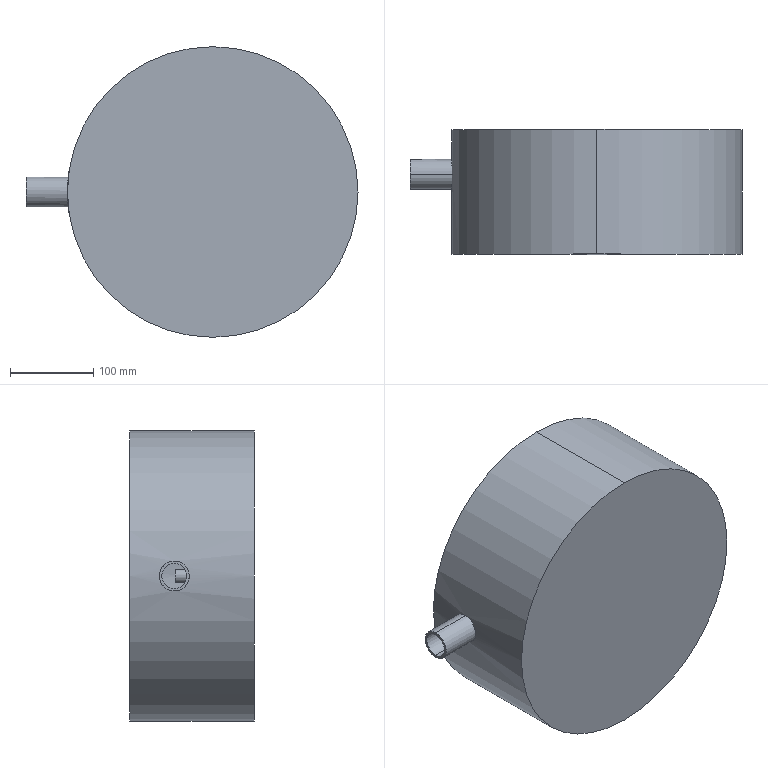Part | SolidWorks | features ICE 6, Extrusion 1, Shell 1 | 1 solid | 36 faces | box 400 x 150 x 350 mm | volume 1908298 mm3 | cylinder 24 | plane 12 | commonest cylinder face diameters 5 x8 36 x4 16 x2 30 x2 120 x2 320 x2
STEP:
#1=CARTESIAN_POINT('',(0.,145.,167.5));
#2=VERTEX_POINT('',#1);
#3=CARTESIAN_POINT('',(-2.5,145.,169.982));
#4=VERTEX_POINT('',#3);
#5=CARTESIAN_POINT('',(0.,145.,170.));
#6=DIRECTION('',(0.,1.,0.));
#7=DIRECTION('',(0.,0.,1.));
#8=AXIS2_PLACEMENT_3D('',#5,#6,#7);
#9=CIRCLE('',#8,2.5);
#10=EDGE_CURVE('',#2,#4,#9,.T.);
#11=ORIENTED_EDGE('',*,*,#10,.F.);
#12=CARTESIAN_POINT('',(0.,150.,167.5));
#13=VERTEX_POINT('',#12);
#14=CARTESIAN_POINT('',(0.,140.,167.5));
#15=DIRECTION('',(0.,1.,0.));
#16=VECTOR('',#15,1000.);
#17=LINE('',#14,#16);
#18=EDGE_CURVE('',#2,#13,#17,.T.);
#19=ORIENTED_EDGE('',*,*,#18,.T.);
#20=CARTESIAN_POINT('',(0.,150.,172.5));
#21=VERTEX_POINT('',#20);
#22=CARTESIAN_POINT('',(0.,150.,170.));
#23=DIRECTION('',(0.,1.,0.));
#24=DIRECTION('',(0.,0.,1.));
#25=AXIS2_PLACEMENT_3D('',#22,#23,#24);
#26=CIRCLE('',#25,2.5);
#27=EDGE_CURVE('',#13,#21,#26,.T.);
#28=ORIENTED_EDGE('',*,*,#27,.T.);
#29=CARTESIAN_POINT('',(0.,140.,172.5));
#30=VERTEX_POINT('',#29);
#31=CARTESIAN_POINT('',(0.,140.,172.5));
#32=DIRECTION('',(0.,1.,0.));
#33=VECTOR('',#32,1000.);
#34=LINE('',#31,#33);
#35=EDGE_CURVE('',#30,#21,#34,.T.);
#36=ORIENTED_EDGE('',*,*,#35,.F.);
#37=CARTESIAN_POINT('',(-2.5,140.,169.982));
#38=VERTEX_POINT('',#37);
#39=CARTESIAN_POINT('',(0.,140.,170.));
#40=DIRECTION('',(0.,1.,0.));
#41=DIRECTION('',(0.,0.,1.));
#42=AXIS2_PLACEMENT_3D('',#39,#40,#41);
#43=CIRCLE('',#42,2.5);
#44=EDGE_CURVE('',#38,#30,#43,.T.);
#45=ORIENTED_EDGE('',*,*,#44,.F.);
#46=CARTESIAN_POINT('',(-2.5,145.,169.982));
#47=DIRECTION('',(0.,1.,0.));
#48=VECTOR('',#47,1000.);
#49=LINE('',#46,#48);
#50=EDGE_CURVE('',#38,#4,#49,.T.);
#51=ORIENTED_EDGE('',*,*,#50,.T.);
#52=EDGE_LOOP('',(#11,#19,#28,#36,#45,#51));
#53=FACE_OUTER_BOUND('',#52,.T.);
#54=CARTESIAN_POINT('',(0.,140.,170.));
#55=DIRECTION('',(0.,1.,0.));
#56=DIRECTION('',(0.,0.,1.));
#57=AXIS2_PLACEMENT_3D('',#54,#55,#56);
#58=CYLINDRICAL_SURFACE('',#57,2.5);
#59=ADVANCED_FACE('',(#53),#58,.F.);
#60=CARTESIAN_POINT('',(-170.,140.,-2.5));
#61=VERTEX_POINT('',#60);
#62=CARTESIAN_POINT('',(-170.,140.,2.5));
#63=VERTEX_POINT('',#62);
#64=CARTESIAN_POINT('',(-170.,140.,0.));
#65=DIRECTION('',(0.,1.,0.));
#66=DIRECTION('',(0.,0.,1.));
#67=AXIS2_PLACEMENT_3D('',#64,#65,#66);
#68=CIRCLE('',#67,2.5);
#69=EDGE_CURVE('',#61,#63,#68,.T.);
#70=ORIENTED_EDGE('',*,*,#69,.F.);
#71=CARTESIAN_POINT('',(-170.,150.,-2.5));
#72=VERTEX_POINT('',#71);
#73=CARTESIAN_POINT('',(-170.,140.,-2.5));
#74=DIRECTION('',(0.,1.,0.));
#75=VECTOR('',#74,1000.);
#76=LINE('',#73,#75);
#77=EDGE_CURVE('',#61,#72,#76,.T.);
#78=ORIENTED_EDGE('',*,*,#77,.T.);
#79=CARTESIAN_POINT('',(-170.,150.,2.5));
#80=VERTEX_POINT('',#79);
#81=CARTESIAN_POINT('',(-170.,150.,0.));
#82=DIRECTION('',(0.,1.,0.));
#83=DIRECTION('',(0.,0.,1.));
#84=AXIS2_PLACEMENT_3D('',#81,#82,#83);
#85=CIRCLE('',#84,2.5);
#86=EDGE_CURVE('',#72,#80,#85,.T.);
#87=ORIENTED_EDGE('',*,*,#86,.T.);
#88=CARTESIAN_POINT('',(-170.,140.,2.5));
#89=DIRECTION('',(0.,1.,0.));
#90=VECTOR('',#89,1000.);
#91=LINE('',#88,#90);
#92=EDGE_CURVE('',#63,#80,#91,.T.);
#93=ORIENTED_EDGE('',*,*,#92,.F.);
#94=EDGE_LOOP('',(#70,#78,#87,#93));
#95=FACE_OUTER_BOUND('',#94,.T.);
#96=CARTESIAN_POINT('',(-170.,140.,0.));
#97=DIRECTION('',(0.,1.,0.));
#98=DIRECTION('',(0.,0.,1.));
#99=AXIS2_PLACEMENT_3D('',#96,#97,#98);
#100=CYLINDRICAL_SURFACE('',#99,2.5);
#101=ADVANCED_FACE('',(#95),#100,.F.);
#102=CARTESIAN_POINT('',(0.,140.,-172.5));
#103=VERTEX_POINT('',#102);
#104=CARTESIAN_POINT('',(-2.5,140.,-169.982));
#105=VERTEX_POINT('',#104);
#106=CARTESIAN_POINT('',(0.,140.,-170.));
#107=DIRECTION('',(0.,1.,0.));
#108=DIRECTION('',(0.,0.,1.));
#109=AXIS2_PLACEMENT_3D('',#106,#107,#108);
#110=CIRCLE('',#109,2.5);
#111=EDGE_CURVE('',#103,#105,#110,.T.);
#112=ORIENTED_EDGE('',*,*,#111,.F.);
#113=CARTESIAN_POINT('',(0.,150.,-172.5));
#114=VERTEX_POINT('',#113);
#115=CARTESIAN_POINT('',(0.,140.,-172.5));
#116=DIRECTION('',(0.,1.,0.));
#117=VECTOR('',#116,1000.);
#118=LINE('',#115,#117);
#119=EDGE_CURVE('',#103,#114,#118,.T.);
#120=ORIENTED_EDGE('',*,*,#119,.T.);
#121=CARTESIAN_POINT('',(0.,150.,-167.5));
#122=VERTEX_POINT('',#121);
#123=CARTESIAN_POINT('',(0.,150.,-170.));
#124=DIRECTION('',(0.,1.,0.));
#125=DIRECTION('',(0.,0.,1.));
#126=AXIS2_PLACEMENT_3D('',#123,#124,#125);
#127=CIRCLE('',#126,2.5);
#128=EDGE_CURVE('',#114,#122,#127,.T.);
#129=ORIENTED_EDGE('',*,*,#128,.T.);
#130=CARTESIAN_POINT('',(0.,145.,-167.5));
#131=VERTEX_POINT('',#130);
#132=CARTESIAN_POINT('',(0.,140.,-167.5));
#133=DIRECTION('',(0.,1.,0.));
#134=VECTOR('',#133,1000.);
#135=LINE('',#132,#134);
#136=EDGE_CURVE('',#131,#122,#135,.T.);
#137=ORIENTED_EDGE('',*,*,#136,.F.);
#138=CARTESIAN_POINT('',(-2.5,145.,-169.982));
#139=VERTEX_POINT('',#138);
#140=CARTESIAN_POINT('',(0.,145.,-170.));
#141=DIRECTION('',(0.,1.,0.));
#142=DIRECTION('',(0.,0.,1.));
#143=AXIS2_PLACEMENT_3D('',#140,#141,#142);
#144=CIRCLE('',#143,2.5);
#145=EDGE_CURVE('',#139,#131,#144,.T.);
#146=ORIENTED_EDGE('',*,*,#145,.F.);
#147=CARTESIAN_POINT('',(-2.5,145.,-169.982));
#148=DIRECTION('',(0.,-1.,0.));
#149=VECTOR('',#148,1000.);
#150=LINE('',#147,#149);
#151=EDGE_CURVE('',#139,#105,#150,.T.);
#152=ORIENTED_EDGE('',*,*,#151,.T.);
#153=EDGE_LOOP('',(#112,#120,#129,#137,#146,#152));
#154=FACE_OUTER_BOUND('',#153,.T.);
#155=CARTESIAN_POINT('',(0.,140.,-170.));
#156=DIRECTION('',(0.,1.,0.));
#157=DIRECTION('',(0.,0.,1.));
#158=AXIS2_PLACEMENT_3D('',#155,#156,#157);
#159=CYLINDRICAL_SURFACE('',#158,2.5);
#160=ADVANCED_FACE('',(#154),#159,.F.);
#161=CARTESIAN_POINT('',(170.,140.,-2.5));
#162=VERTEX_POINT('',#161);
#163=CARTESIAN_POINT('',(169.982,140.,-2.5));
#164=VERTEX_POINT('',#163);
#165=CARTESIAN_POINT('',(170.,140.,0.));
#166=DIRECTION('',(0.,1.,0.));
#167=DIRECTION('',(0.,0.,1.));
#168=AXIS2_PLACEMENT_3D('',#165,#166,#167);
#169=CIRCLE('',#168,2.5);
#170=EDGE_CURVE('',#162,#164,#169,.T.);
#171=ORIENTED_EDGE('',*,*,#170,.F.);
#172=CARTESIAN_POINT('',(170.,150.,-2.5));
#173=VERTEX_POINT('',#172);
#174=CARTESIAN_POINT('',(170.,140.,-2.5));
#175=DIRECTION('',(0.,1.,0.));
#176=VECTOR('',#175,1000.);
#177=LINE('',#174,#176);
#178=EDGE_CURVE('',#162,#173,#177,.T.);
#179=ORIENTED_EDGE('',*,*,#178,.T.);
#180=CARTESIAN_POINT('',(170.,150.,2.5));
#181=VERTEX_POINT('',#180);
#182=CARTESIAN_POINT('',(170.,150.,0.));
#183=DIRECTION('',(0.,1.,0.));
#184=DIRECTION('',(0.,0.,1.));
#185=AXIS2_PLACEMENT_3D('',#182,#183,#184);
#186=CIRCLE('',#185,2.5);
#187=EDGE_CURVE('',#173,#181,#186,.T.);
#188=ORIENTED_EDGE('',*,*,#187,.T.);
#189=CARTESIAN_POINT('',(170.,140.,2.5));
#190=VERTEX_POINT('',#189);
#191=CARTESIAN_POINT('',(170.,140.,2.5));
#192=DIRECTION('',(0.,1.,0.));
#193=VECTOR('',#192,1000.);
#194=LINE('',#191,#193);
#195=EDGE_CURVE('',#190,#181,#194,.T.);
#196=ORIENTED_EDGE('',*,*,#195,.F.);
#197=CARTESIAN_POINT('',(169.982,140.,2.5));
#198=VERTEX_POINT('',#197);
#199=CARTESIAN_POINT('',(170.,140.,0.));
#200=DIRECTION('',(0.,1.,0.));
#201=DIRECTION('',(0.,0.,1.));
#202=AXIS2_PLACEMENT_3D('',#199,#200,#201);
#203=CIRCLE('',#202,2.5);
#204=EDGE_CURVE('',#198,#190,#203,.T.);
#205=ORIENTED_EDGE('',*,*,#204,.F.);
#206=CARTESIAN_POINT('',(169.982,145.,2.5));
#207=VERTEX_POINT('',#206);
#208=CARTESIAN_POINT('',(169.982,145.,2.5));
#209=DIRECTION('',(0.,1.,0.));
#210=VECTOR('',#209,1000.);
#211=LINE('',#208,#210);
#212=EDGE_CURVE('',#198,#207,#211,.T.);
#213=ORIENTED_EDGE('',*,*,#212,.T.);
#214=CARTESIAN_POINT('',(169.982,145.,-2.5));
#215=VERTEX_POINT('',#214);
#216=CARTESIAN_POINT('',(170.,145.,0.));
#217=DIRECTION('',(0.,1.,0.));
#218=DIRECTION('',(0.,0.,1.));
#219=AXIS2_PLACEMENT_3D('',#216,#217,#218);
#220=CIRCLE('',#219,2.5);
#221=EDGE_CURVE('',#215,#207,#220,.T.);
#222=ORIENTED_EDGE('',*,*,#221,.F.);
#223=CARTESIAN_POINT('',(169.982,145.,-2.5));
#224=DIRECTION('',(0.,-1.,0.));
#225=VECTOR('',#224,1000.);
#226=LINE('',#223,#225);
#227=EDGE_CURVE('',#215,#164,#226,.T.);
#228=ORIENTED_EDGE('',*,*,#227,.T.);
#229=EDGE_LOOP('',(#171,#179,#188,#196,#205,#213,#222,#228));
#230=FACE_OUTER_BOUND('',#229,.T.);
#231=CARTESIAN_POINT('',(170.,140.,0.));
#232=DIRECTION('',(0.,1.,0.));
#233=DIRECTION('',(0.,0.,1.));
#234=AXIS2_PLACEMENT_3D('',#231,#232,#233);
#235=CYLINDRICAL_SURFACE('',#234,2.5);
#236=ADVANCED_FACE('',(#230),#235,.F.);
#237=CARTESIAN_POINT('',(0.,145.,-160.));
#238=VERTEX_POINT('',#237);
#239=CARTESIAN_POINT('',(0.,145.,160.));
#240=VERTEX_POINT('',#239);
#241=CARTESIAN_POINT('',(0.,145.,0.));
#242=DIRECTION('',(0.,1.,0.));
#243=DIRECTION('',(0.,0.,1.));
#244=AXIS2_PLACEMENT_3D('',#241,#242,#243);
#245=CIRCLE('',#244,160.);
#246=EDGE_CURVE('',#238,#240,#245,.T.);
#247=ORIENTED_EDGE('',*,*,#246,.F.);
#248=CARTESIAN_POINT('',(0.,150.,-160.));
#249=VERTEX_POINT('',#248);
#250=CARTESIAN_POINT('',(0.,145.,-160.));
#251=DIRECTION('',(0.,1.,0.));
#252=VECTOR('',#251,1000.);
#253=LINE('',#250,#252);
#254=EDGE_CURVE('',#238,#249,#253,.T.);
#255=ORIENTED_EDGE('',*,*,#254,.T.);
#256=CARTESIAN_POINT('',(0.,150.,160.));
#257=VERTEX_POINT('',#256);
#258=CARTESIAN_POINT('',(0.,150.,0.));
#259=DIRECTION('',(0.,1.,0.));
#260=DIRECTION('',(0.,0.,1.));
#261=AXIS2_PLACEMENT_3D('',#258,#259,#260);
#262=CIRCLE('',#261,160.);
#263=EDGE_CURVE('',#249,#257,#262,.T.);
#264=ORIENTED_EDGE('',*,*,#263,.T.);
#265=CARTESIAN_POINT('',(0.,145.,160.));
#266=DIRECTION('',(0.,1.,0.));
#267=VECTOR('',#266,1000.);
#268=LINE('',#265,#267);
#269=EDGE_CURVE('',#240,#257,#268,.T.);
#270=ORIENTED_EDGE('',*,*,#269,.F.);
#271=EDGE_LOOP('',(#247,#255,#264,#270));
#272=FACE_OUTER_BOUND('',#271,.T.);
#273=CARTESIAN_POINT('',(0.,145.,0.));
#274=DIRECTION('',(0.,1.,0.));
#275=DIRECTION('',(0.,0.,1.));
#276=AXIS2_PLACEMENT_3D('',#273,#274,#275);
#277=CYLINDRICAL_SURFACE('',#276,160.);
#278=ADVANCED_FACE('',(#272),#277,.F.);
#279=CARTESIAN_POINT('',(0.,95.,8.));
#280=VERTEX_POINT('',#279);
#281=CARTESIAN_POINT('',(0.,95.,-8.));
#282=VERTEX_POINT('',#281);
#283=CARTESIAN_POINT('',(0.,95.,0.));
#284=DIRECTION('',(0.,1.,0.));
#285=DIRECTION('',(0.,0.,1.));
#286=AXIS2_PLACEMENT_3D('',#283,#284,#285);
#287=CIRCLE('',#286,8.);
#288=EDGE_CURVE('',#280,#282,#287,.T.);
#289=ORIENTED_EDGE('',*,*,#288,.F.);
#290=CARTESIAN_POINT('',(0.,55.,8.));
#291=VERTEX_POINT('',#290);
#292=CARTESIAN_POINT('',(0.,95.,8.));
#293=DIRECTION('',(0.,-1.,0.));
#294=VECTOR('',#293,1000.);
#295=LINE('',#292,#294);
#296=EDGE_CURVE('',#280,#291,#295,.T.);
#297=ORIENTED_EDGE('',*,*,#296,.T.);
#298=CARTESIAN_POINT('',(0.,55.,-8.));
#299=VERTEX_POINT('',#298);
#300=CARTESIAN_POINT('',(0.,55.,0.));
#301=DIRECTION('',(0.,1.,0.));
#302=DIRECTION('',(0.,0.,1.));
#303=AXIS2_PLACEMENT_3D('',#300,#301,#302);
#304=CIRCLE('',#303,8.);
#305=EDGE_CURVE('',#291,#299,#304,.T.);
#306=ORIENTED_EDGE('',*,*,#305,.T.);
#307=CARTESIAN_POINT('',(0.,95.,-8.));
#308=DIRECTION('',(0.,-1.,0.));
#309=VECTOR('',#308,1000.);
#310=LINE('',#307,#309);
#311=EDGE_CURVE('',#282,#299,#310,.T.);
#312=ORIENTED_EDGE('',*,*,#311,.F.);
#313=EDGE_LOOP('',(#289,#297,#306,#312));
#314=FACE_OUTER_BOUND('',#313,.T.);
#315=CARTESIAN_POINT('',(0.,95.,0.));
#316=DIRECTION('',(0.,-1.,0.));
#317=DIRECTION('',(0.,0.,-1.));
#318=AXIS2_PLACEMENT_3D('',#315,#316,#317);
#319=CYLINDRICAL_SURFACE('',#318,8.);
#320=ADVANCED_FACE('',(#314),#319,.T.);
#321=CARTESIAN_POINT('',(-155.,96.363,-15.));
#322=VERTEX_POINT('',#321);
#323=CARTESIAN_POINT('',(-155.,96.363,15.));
#324=VERTEX_POINT('',#323);
#325=CARTESIAN_POINT('',(-155.,96.363,0.));
#326=DIRECTION('',(-1.,0.,0.));
#327=DIRECTION('',(0.,0.,1.));
#328=AXIS2_PLACEMENT_3D('',#325,#326,#327);
#329=CIRCLE('',#328,15.);
#330=EDGE_CURVE('',#322,#324,#329,.T.);
#331=ORIENTED_EDGE('',*,*,#330,.F.);
#332=CARTESIAN_POINT('',(-225.,96.363,-15.));
#333=VERTEX_POINT('',#332);
#334=CARTESIAN_POINT('',(-125.,96.363,-15.));
#335=DIRECTION('',(-1.,0.,0.));
#336=VECTOR('',#335,1000.);
#337=LINE('',#334,#336);
#338=EDGE_CURVE('',#322,#333,#337,.T.);
#339=ORIENTED_EDGE('',*,*,#338,.T.);
#340=CARTESIAN_POINT('',(-225.,96.363,15.));
#341=VERTEX_POINT('',#340);
#342=CARTESIAN_POINT('',(-225.,96.363,0.));
#343=DIRECTION('',(-1.,0.,0.));
#344=DIRECTION('',(0.,0.,1.));
#345=AXIS2_PLACEMENT_3D('',#342,#343,#344);
#346=CIRCLE('',#345,15.);
#347=EDGE_CURVE('',#333,#341,#346,.T.);
#348=ORIENTED_EDGE('',*,*,#347,.T.);
#349=CARTESIAN_POINT('',(-125.,96.363,15.));
#350=DIRECTION('',(-1.,0.,0.));
#351=VECTOR('',#350,1000.);
#352=LINE('',#349,#351);
#353=EDGE_CURVE('',#324,#341,#352,.T.);
#354=ORIENTED_EDGE('',*,*,#353,.F.);
#355=EDGE_LOOP('',(#331,#339,#348,#354));
#356=FACE_OUTER_BOUND('',#355,.T.);
#357=CARTESIAN_POINT('',(-125.,96.363,0.));
#358=DIRECTION('',(-1.,0.,0.));
#359=DIRECTION('',(0.,0.,1.));
#360=AXIS2_PLACEMENT_3D('',#357,#358,#359);
#361=CYLINDRICAL_SURFACE('',#360,15.);
#362=ADVANCED_FACE('',(#356),#361,.F.);
#363=CARTESIAN_POINT('',(-174.072,96.363,-18.));
#364=VERTEX_POINT('',#363);
#365=CARTESIAN_POINT('',(-174.072,96.363,18.));
#366=VERTEX_POINT('',#365);
#367=CARTESIAN_POINT('',(-174.072,96.363,-18.));
#368=CARTESIAN_POINT('',(-174.072,97.538,-18.));
#369=CARTESIAN_POINT('',(-174.084,98.706,-17.886));
#370=CARTESIAN_POINT('',(-174.119,100.448,-17.54));
#371=CARTESIAN_POINT('',(-174.133,101.027,-17.395));
#372=CARTESIAN_POINT('',(-174.167,102.154,-17.053));
#373=CARTESIAN_POINT('',(-174.187,102.707,-16.855));
#374=CARTESIAN_POINT('',(-174.229,103.79,-16.407));
#375=CARTESIAN_POINT('',(-174.253,104.32,-16.156));
#376=CARTESIAN_POINT('',(-174.303,105.359,-15.602));
#377=CARTESIAN_POINT('',(-174.331,105.87,-15.296));
#378=CARTESIAN_POINT('',(-174.415,107.346,-14.31));
#379=CARTESIAN_POINT('',(-174.475,108.252,-13.566));
#380=CARTESIAN_POINT('',(-174.566,109.497,-12.322));
#381=CARTESIAN_POINT('',(-174.596,109.893,-11.886));
#382=CARTESIAN_POINT('',(-174.656,110.646,-10.97));
#383=CARTESIAN_POINT('',(-174.686,111.,-10.494));
#384=CARTESIAN_POINT('',(-174.77,111.98,-9.028));
#385=CARTESIAN_POINT('',(-174.821,112.533,-7.995));
#386=CARTESIAN_POINT('',(-174.885,113.212,-6.361));
#387=CARTESIAN_POINT('',(-174.905,113.413,-5.8));
#388=CARTESIAN_POINT('',(-174.939,113.757,-4.668));
#389=CARTESIAN_POINT('',(-174.953,113.9,-4.098));
#390=CARTESIAN_POINT('',(-174.988,114.245,-2.372));
#391=CARTESIAN_POINT('',(-175.,114.362,-1.203));
#392=CARTESIAN_POINT('',(-175.,114.364,1.176));
#393=CARTESIAN_POINT('',(-174.988,114.248,2.347));
#394=CARTESIAN_POINT('',(-174.954,113.906,4.073));
#395=CARTESIAN_POINT('',(-174.939,113.764,4.644));
#396=CARTESIAN_POINT('',(-174.906,113.422,5.775));
#397=CARTESIAN_POINT('',(-174.886,113.221,6.337));
#398=CARTESIAN_POINT('',(-174.822,112.544,7.972));
#399=CARTESIAN_POINT('',(-174.771,111.992,9.006));
#400=CARTESIAN_POINT('',(-174.687,111.014,10.474));
#401=CARTESIAN_POINT('',(-174.658,110.662,10.95));
#402=CARTESIAN_POINT('',(-174.598,109.91,11.867));
#403=CARTESIAN_POINT('',(-174.567,109.514,12.304));
#404=CARTESIAN_POINT('',(-174.477,108.271,13.549));
#405=CARTESIAN_POINT('',(-174.416,107.366,14.295));
#406=CARTESIAN_POINT('',(-174.332,105.892,15.282));
#407=CARTESIAN_POINT('',(-174.304,105.381,15.589));
#408=CARTESIAN_POINT('',(-174.254,104.343,16.145));
#409=CARTESIAN_POINT('',(-174.23,103.813,16.397));
#410=CARTESIAN_POINT('',(-174.187,102.731,16.846));
#411=CARTESIAN_POINT('',(-174.168,102.178,17.045));
#412=CARTESIAN_POINT('',(-174.134,101.052,17.389));
#413=CARTESIAN_POINT('',(-174.119,100.475,17.534));
#414=CARTESIAN_POINT('',(-174.084,98.73,17.883));
#415=CARTESIAN_POINT('',(-174.072,97.553,18.));
#416=CARTESIAN_POINT('',(-174.072,96.363,18.));
#417=B_SPLINE_CURVE_WITH_KNOTS('',3,(#367,#368,#369,#370,#371,#372,#373,#374,#375,#376,#377,#378,#379,#380,#381,#382,#383,#384,#385,#386,#387,#388,#389,#390,#391,#392,#393,#394,#395,#396,#397,#398,#399,#400,#401,#402,#403,#404,#405,#406,#407,#408,#409,#410,#411,#412,#413,#414,#415,#416),.UNSPECIFIED.,.F.,.F.,(4,2,2,2,2,2,2,2,2,2,2,2,2,2,2,2,2,2,2,2,2,2,2,2,4),(0.05631,0.05983,0.06159,0.06335,0.06511,0.06687,0.07039,0.07215,0.07391,0.07743,0.07919,0.08094,0.08446,0.08798,0.08974,0.0915,0.09502,0.09678,0.09854,0.1021,0.1038,0.1056,0.1073,0.1091,0.1126),.UNSPECIFIED.);
#418=EDGE_CURVE('',#364,#366,#417,.T.);
#419=ORIENTED_EDGE('',*,*,#418,.F.);
#420=CARTESIAN_POINT('',(-225.,96.363,-18.));
#421=VERTEX_POINT('',#420);
#422=CARTESIAN_POINT('',(-155.,96.363,-18.));
#423=DIRECTION('',(-1.,0.,0.));
#424=VECTOR('',#423,1000.);
#425=LINE('',#422,#424);
#426=EDGE_CURVE('',#364,#421,#425,.T.);
#427=ORIENTED_EDGE('',*,*,#426,.T.);
#428=CARTESIAN_POINT('',(-225.,96.363,18.));
#429=VERTEX_POINT('',#428);
#430=CARTESIAN_POINT('',(-225.,96.363,0.));
#431=DIRECTION('',(-1.,0.,0.));
#432=DIRECTION('',(0.,0.,1.));
#433=AXIS2_PLACEMENT_3D('',#430,#431,#432);
#434=CIRCLE('',#433,18.);
#435=EDGE_CURVE('',#429,#421,#434,.T.);
#436=ORIENTED_EDGE('',*,*,#435,.F.);
#437=CARTESIAN_POINT('',(-155.,96.363,18.));
#438=DIRECTION('',(-1.,0.,0.));
#439=VECTOR('',#438,1000.);
#440=LINE('',#437,#439);
#441=EDGE_CURVE('',#366,#429,#440,.T.);
#442=ORIENTED_EDGE('',*,*,#441,.F.);
#443=EDGE_LOOP('',(#419,#427,#436,#442));
#444=FACE_OUTER_BOUND('',#443,.T.);
#445=CARTESIAN_POINT('',(-155.,96.363,0.));
#446=DIRECTION('',(-1.,0.,0.));
#447=DIRECTION('',(0.,0.,1.));
#448=AXIS2_PLACEMENT_3D('',#445,#446,#447);
#449=CYLINDRICAL_SURFACE('',#448,18.);
#450=ADVANCED_FACE('',(#444),#449,.T.);
#451=CARTESIAN_POINT('',(-155.,96.363,18.));
#452=VERTEX_POINT('',#451);
#453=CARTESIAN_POINT('',(-155.,96.363,-18.));
#454=VERTEX_POINT('',#453);
#455=CARTESIAN_POINT('',(-155.,96.363,0.));
#456=DIRECTION('',(-1.,0.,0.));
#457=DIRECTION('',(0.,0.,1.));
#458=AXIS2_PLACEMENT_3D('',#455,#456,#457);
#459=CIRCLE('',#458,18.);
#460=EDGE_CURVE('',#452,#454,#459,.T.);
#461=ORIENTED_EDGE('',*,*,#460,.T.);
#462=CARTESIAN_POINT('',(-169.044,96.363,-18.));
#463=VERTEX_POINT('',#462);
#464=CARTESIAN_POINT('',(-155.,96.363,-18.));
#465=DIRECTION('',(-1.,0.,0.));
#466=VECTOR('',#465,1000.);
#467=LINE('',#464,#466);
#468=EDGE_CURVE('',#454,#463,#467,.T.);
#469=ORIENTED_EDGE('',*,*,#468,.T.);
#470=CARTESIAN_POINT('',(-169.044,96.363,18.));
#471=VERTEX_POINT('',#470);
#472=CARTESIAN_POINT('',(-169.044,96.363,-18.));
#473=CARTESIAN_POINT('',(-169.044,97.538,-18.));
#474=CARTESIAN_POINT('',(-169.057,98.706,-17.886));
#475=CARTESIAN_POINT('',(-169.093,100.449,-17.54));
#476=CARTESIAN_POINT('',(-169.108,101.027,-17.395));
#477=CARTESIAN_POINT('',(-169.143,102.154,-17.053));
#478=CARTESIAN_POINT('',(-169.163,102.707,-16.855));
#479=CARTESIAN_POINT('',(-169.207,103.79,-16.407));
#480=CARTESIAN_POINT('',(-169.231,104.321,-16.156));
#481=CARTESIAN_POINT('',(-169.283,105.359,-15.602));
#482=CARTESIAN_POINT('',(-169.311,105.87,-15.296));
#483=CARTESIAN_POINT('',(-169.398,107.346,-14.31));
#484=CARTESIAN_POINT('',(-169.46,108.252,-13.566));
#485=CARTESIAN_POINT('',(-169.553,109.497,-12.322));
#486=CARTESIAN_POINT('',(-169.585,109.893,-11.886));
#487=CARTESIAN_POINT('',(-169.646,110.646,-10.97));
#488=CARTESIAN_POINT('',(-169.677,110.999,-10.494));
#489=CARTESIAN_POINT('',(-169.763,111.98,-9.028));
#490=CARTESIAN_POINT('',(-169.815,112.533,-7.995));
#491=CARTESIAN_POINT('',(-169.882,113.212,-6.361));
#492=CARTESIAN_POINT('',(-169.902,113.413,-5.8));
#493=CARTESIAN_POINT('',(-169.937,113.757,-4.669));
#494=CARTESIAN_POINT('',(-169.952,113.9,-4.098));
#495=CARTESIAN_POINT('',(-169.987,114.245,-2.372));
#496=CARTESIAN_POINT('',(-170.,114.362,-1.203));
#497=CARTESIAN_POINT('',(-170.,114.364,1.176));
#498=CARTESIAN_POINT('',(-169.988,114.248,2.347));
#499=CARTESIAN_POINT('',(-169.952,113.906,4.073));
#500=CARTESIAN_POINT('',(-169.938,113.764,4.644));
#501=CARTESIAN_POINT('',(-169.903,113.422,5.775));
#502=CARTESIAN_POINT('',(-169.883,113.221,6.337));
#503=CARTESIAN_POINT('',(-169.816,112.544,7.972));
#504=CARTESIAN_POINT('',(-169.764,111.992,9.006));
#505=CARTESIAN_POINT('',(-169.678,111.014,10.474));
#506=CARTESIAN_POINT('',(-169.648,110.661,10.95));
#507=CARTESIAN_POINT('',(-169.586,109.91,11.868));
#508=CARTESIAN_POINT('',(-169.555,109.514,12.304));
#509=CARTESIAN_POINT('',(-169.461,108.271,13.549));
#510=CARTESIAN_POINT('',(-169.399,107.366,14.295));
#511=CARTESIAN_POINT('',(-169.312,105.892,15.282));
#512=CARTESIAN_POINT('',(-169.284,105.381,15.589));
#513=CARTESIAN_POINT('',(-169.232,104.343,16.145));
#514=CARTESIAN_POINT('',(-169.208,103.813,16.396));
#515=CARTESIAN_POINT('',(-169.163,102.731,16.846));
#516=CARTESIAN_POINT('',(-169.143,102.179,17.045));
#517=CARTESIAN_POINT('',(-169.108,101.052,17.388));
#518=CARTESIAN_POINT('',(-169.093,100.475,17.534));
#519=CARTESIAN_POINT('',(-169.057,98.73,17.883));
#520=CARTESIAN_POINT('',(-169.044,97.553,18.));
#521=CARTESIAN_POINT('',(-169.044,96.363,18.));
#522=B_SPLINE_CURVE_WITH_KNOTS('',3,(#472,#473,#474,#475,#476,#477,#478,#479,#480,#481,#482,#483,#484,#485,#486,#487,#488,#489,#490,#491,#492,#493,#494,#495,#496,#497,#498,#499,#500,#501,#502,#503,#504,#505,#506,#507,#508,#509,#510,#511,#512,#513,#514,#515,#516,#517,#518,#519,#520,#521),.UNSPECIFIED.,.F.,.F.,(4,2,2,2,2,2,2,2,2,2,2,2,2,2,2,2,2,2,2,2,2,2,2,2,4),(0.05632,0.05983,0.06159,0.06335,0.06511,0.06687,0.07039,0.07215,0.07391,0.07743,0.07919,0.08095,0.08447,0.08799,0.08975,0.0915,0.09502,0.09678,0.09854,0.1021,0.1038,0.1056,0.1073,0.1091,0.1126),.UNSPECIFIED.);
#523=EDGE_CURVE('',#463,#471,#522,.T.);
#524=ORIENTED_EDGE('',*,*,#523,.T.);
#525=CARTESIAN_POINT('',(-155.,96.363,18.));
#526=DIRECTION('',(-1.,0.,0.));
#527=VECTOR('',#526,1000.);
#528=LINE('',#525,#527);
#529=EDGE_CURVE('',#452,#471,#528,.T.);
#530=ORIENTED_EDGE('',*,*,#529,.F.);
#531=EDGE_LOOP('',(#461,#469,#524,#530));
#532=FACE_OUTER_BOUND('',#531,.T.);
#533=CARTESIAN_POINT('',(-155.,96.363,0.));
#534=DIRECTION('',(-1.,0.,0.));
#535=DIRECTION('',(0.,0.,1.));
#536=AXIS2_PLACEMENT_3D('',#533,#534,#535);
#537=CYLINDRICAL_SURFACE('',#536,18.);
#538=ADVANCED_FACE('',(#532),#537,.T.);
#539=CARTESIAN_POINT('',(0.,55.,60.));
#540=VERTEX_POINT('',#539);
#541=CARTESIAN_POINT('',(0.,55.,-60.));
#542=VERTEX_POINT('',#541);
#543=CARTESIAN_POINT('',(0.,55.,0.));
#544=DIRECTION('',(0.,1.,0.));
#545=DIRECTION('',(0.,0.,1.));
#546=AXIS2_PLACEMENT_3D('',#543,#544,#545);
#547=CIRCLE('',#546,60.);
#548=EDGE_CURVE('',#540,#542,#547,.T.);
#549=ORIENTED_EDGE('',*,*,#548,.F.);
#550=CARTESIAN_POINT('',(0.,5.,60.));
#551=VERTEX_POINT('',#550);
#552=CARTESIAN_POINT('',(0.,55.,60.));
#553=DIRECTION('',(0.,-1.,0.));
#554=VECTOR('',#553,1000.);
#555=LINE('',#552,#554);
#556=EDGE_CURVE('',#540,#551,#555,.T.);
#557=ORIENTED_EDGE('',*,*,#556,.T.);
#558=CARTESIAN_POINT('',(0.,5.,-60.));
#559=VERTEX_POINT('',#558);
#560=CARTESIAN_POINT('',(0.,5.,0.));
#561=DIRECTION('',(0.,1.,0.));
#562=DIRECTION('',(0.,0.,1.));
#563=AXIS2_PLACEMENT_3D('',#560,#561,#562);
#564=CIRCLE('',#563,60.);
#565=EDGE_CURVE('',#551,#559,#564,.T.);
#566=ORIENTED_EDGE('',*,*,#565,.T.);
#567=CARTESIAN_POINT('',(0.,55.,-60.));
#568=DIRECTION('',(0.,-1.,0.));
#569=VECTOR('',#568,1000.);
#570=LINE('',#567,#569);
#571=EDGE_CURVE('',#542,#559,#570,.T.);
#572=ORIENTED_EDGE('',*,*,#571,.F.);
#573=EDGE_LOOP('',(#549,#557,#566,#572));
#574=FACE_OUTER_BOUND('',#573,.T.);
#575=CARTESIAN_POINT('',(0.,55.,0.));
#576=DIRECTION('',(0.,-1.,0.));
#577=DIRECTION('',(0.,0.,-1.));
#578=AXIS2_PLACEMENT_3D('',#575,#576,#577);
#579=CYLINDRICAL_SURFACE('',#578,60.);
#580=ADVANCED_FACE('',(#574),#579,.T.);
#581=CARTESIAN_POINT('',(0.,150.,175.));
#582=VERTEX_POINT('',#581);
#583=CARTESIAN_POINT('',(0.,150.,-175.));
#584=VERTEX_POINT('',#583);
#585=CARTESIAN_POINT('',(0.,150.,0.));
#586=DIRECTION('',(0.,1.,0.));
#587=DIRECTION('',(0.,0.,1.));
#588=AXIS2_PLACEMENT_3D('',#585,#586,#587);
#589=CIRCLE('',#588,175.);
#590=EDGE_CURVE('',#582,#584,#589,.T.);
#591=ORIENTED_EDGE('',*,*,#590,.F.);
#592=CARTESIAN_POINT('',(0.,0.,175.));
#593=VERTEX_POINT('',#592);
#594=CARTESIAN_POINT('',(0.,150.,175.));
#595=DIRECTION('',(0.,-1.,0.));
#596=VECTOR('',#595,1000.);
#597=LINE('',#594,#596);
#598=EDGE_CURVE('',#582,#593,#597,.T.);
#599=ORIENTED_EDGE('',*,*,#598,.T.);
#600=CARTESIAN_POINT('',(0.,0.,-175.));
#601=VERTEX_POINT('',#600);
#602=CARTESIAN_POINT('',(0.,0.,0.));
#603=DIRECTION('',(0.,1.,0.));
#604=DIRECTION('',(0.,0.,1.));
#605=AXIS2_PLACEMENT_3D('',#602,#603,#604);
#606=CIRCLE('',#605,175.);
#607=EDGE_CURVE('',#593,#601,#606,.T.);
#608=ORIENTED_EDGE('',*,*,#607,.T.);
#609=CARTESIAN_POINT('',(0.,150.,-175.));
#610=DIRECTION('',(0.,-1.,0.));
#611=VECTOR('',#610,1000.);
#612=LINE('',#609,#611);
#613=EDGE_CURVE('',#584,#601,#612,.T.);
#614=ORIENTED_EDGE('',*,*,#613,.F.);
#615=EDGE_LOOP('',(#591,#599,#608,#614));
#616=FACE_OUTER_BOUND('',#615,.T.);
#617=CARTESIAN_POINT('',(0.,150.,0.));
#618=DIRECTION('',(0.,-1.,0.));
#619=DIRECTION('',(0.,0.,-1.));
#620=AXIS2_PLACEMENT_3D('',#617,#618,#619);
#621=CYLINDRICAL_SURFACE('',#620,175.);
#622=ADVANCED_FACE('',(#616),#621,.T.);
#623=CARTESIAN_POINT('',(-169.044,96.363,18.));
#624=CARTESIAN_POINT('',(-169.044,95.173,18.));
#625=CARTESIAN_POINT('',(-169.057,94.003,17.883));
#626=CARTESIAN_POINT('',(-169.093,92.276,17.54));
#627=CARTESIAN_POINT('',(-169.108,91.706,17.397));
#628=CARTESIAN_POINT('',(-169.143,90.574,17.054));
#629=CARTESIAN_POINT('',(-169.163,90.012,16.853));
#630=CARTESIAN_POINT('',(-169.229,88.378,16.175));
#631=CARTESIAN_POINT('',(-169.282,87.344,15.622));
#632=CARTESIAN_POINT('',(-169.369,85.877,14.642));
#633=CARTESIAN_POINT('',(-169.399,85.4,14.288));
#634=CARTESIAN_POINT('',(-169.461,84.484,13.536));
#635=CARTESIAN_POINT('',(-169.492,84.048,13.14));
#636=CARTESIAN_POINT('',(-169.585,82.803,11.896));
#637=CARTESIAN_POINT('',(-169.647,82.058,10.99));
#638=CARTESIAN_POINT('',(-169.734,81.071,9.514));
#639=CARTESIAN_POINT('',(-169.762,80.765,9.003));
#640=CARTESIAN_POINT('',(-169.814,80.21,7.964));
#641=CARTESIAN_POINT('',(-169.838,79.959,7.434));
#642=CARTESIAN_POINT('',(-169.882,79.511,6.351));
#643=CARTESIAN_POINT('',(-169.902,79.312,5.799));
#644=CARTESIAN_POINT('',(-169.937,78.97,4.671));
#645=CARTESIAN_POINT('',(-169.952,78.825,4.093));
#646=CARTESIAN_POINT('',(-169.988,78.478,2.35));
#647=CARTESIAN_POINT('',(-170.,78.364,1.181));
#648=CARTESIAN_POINT('',(-170.,78.363,-0.5809));
#649=CARTESIAN_POINT('',(-169.997,78.391,-1.17));
#650=CARTESIAN_POINT('',(-169.985,78.508,-2.351));
#651=CARTESIAN_POINT('',(-169.976,78.595,-2.939));
#652=CARTESIAN_POINT('',(-169.94,78.94,-4.671));
#653=CARTESIAN_POINT('',(-169.905,79.28,-5.794));
#654=CARTESIAN_POINT('',(-169.838,79.957,-7.429));
#655=CARTESIAN_POINT('',(-169.814,80.212,-7.969));
#656=CARTESIAN_POINT('',(-169.762,80.77,-9.01));
#657=CARTESIAN_POINT('',(-169.734,81.072,-9.514));
#658=CARTESIAN_POINT('',(-169.648,82.049,-10.977));
#659=CARTESIAN_POINT('',(-169.586,82.793,-11.886));
#660=CARTESIAN_POINT('',(-169.46,84.474,-13.566));
#661=CARTESIAN_POINT('',(-169.398,85.382,-14.311));
#662=CARTESIAN_POINT('',(-169.311,86.844,-15.288));
#663=CARTESIAN_POINT('',(-169.284,87.348,-15.591));
#664=CARTESIAN_POINT('',(-169.232,88.389,-16.148));
#665=CARTESIAN_POINT('',(-169.207,88.929,-16.404));
#666=CARTESIAN_POINT('',(-169.14,90.564,-17.081));
#667=CARTESIAN_POINT('',(-169.105,91.686,-17.422));
#668=CARTESIAN_POINT('',(-169.069,93.417,-17.767));
#669=CARTESIAN_POINT('',(-169.06,94.004,-17.855));
#670=CARTESIAN_POINT('',(-169.047,95.186,-17.971));
#671=CARTESIAN_POINT('',(-169.044,95.776,-18.));
#672=CARTESIAN_POINT('',(-169.044,96.363,-18.));
#673=B_SPLINE_CURVE_WITH_KNOTS('',3,(#623,#624,#625,#626,#627,#628,#629,#630,#631,#632,#633,#634,#635,#636,#637,#638,#639,#640,#641,#642,#643,#644,#645,#646,#647,#648,#649,#650,#651,#652,#653,#654,#655,#656,#657,#658,#659,#660,#661,#662,#663,#664,#665,#666,#667,#668,#669,#670,#671,#672),.UNSPECIFIED.,.F.,.F.,(4,2,2,2,2,2,2,2,2,2,2,2,2,2,2,2,2,2,2,2,2,2,2,2,4),(0.,0.00352,0.00528,0.007039,0.01056,0.01232,0.01408,0.0176,0.01936,0.02112,0.02288,0.02464,0.02816,0.02992,0.03168,0.0352,0.03696,0.03872,0.04224,0.04576,0.04752,0.04928,0.0528,0.05456,0.05632),.UNSPECIFIED.);
#674=EDGE_CURVE('',#471,#463,#673,.T.);
#675=ORIENTED_EDGE('',*,*,#674,.F.);
#676=ORIENTED_EDGE('',*,*,#523,.F.);
#677=EDGE_LOOP('',(#675,#676));
#678=FACE_BOUND('',#677,.T.);
#679=CARTESIAN_POINT('',(0.,140.,170.));
#680=VERTEX_POINT('',#679);
#681=CARTESIAN_POINT('',(0.,140.,0.));
#682=DIRECTION('',(0.,1.,0.));
#683=DIRECTION('',(0.,0.,1.));
#684=AXIS2_PLACEMENT_3D('',#681,#682,#683);
#685=CIRCLE('',#684,170.);
#686=EDGE_CURVE('',#38,#680,#685,.T.);
#687=ORIENTED_EDGE('',*,*,#686,.T.);
#688=CARTESIAN_POINT('',(0.,5.,170.));
#689=VERTEX_POINT('',#688);
#690=CARTESIAN_POINT('',(0.,150.,170.));
#691=DIRECTION('',(0.,-1.,0.));
#692=VECTOR('',#691,1000.);
#693=LINE('',#690,#692);
#694=EDGE_CURVE('',#680,#689,#693,.T.);
#695=ORIENTED_EDGE('',*,*,#694,.T.);
#696=CARTESIAN_POINT('',(0.,5.,-170.));
#697=VERTEX_POINT('',#696);
#698=CARTESIAN_POINT('',(0.,5.,0.));
#699=DIRECTION('',(0.,1.,0.));
#700=DIRECTION('',(0.,0.,1.));
#701=AXIS2_PLACEMENT_3D('',#698,#699,#700);
#702=CIRCLE('',#701,170.);
#703=EDGE_CURVE('',#697,#689,#702,.T.);
#704=ORIENTED_EDGE('',*,*,#703,.F.);
#705=CARTESIAN_POINT('',(0.,140.,-170.));
#706=VERTEX_POINT('',#705);
#707=CARTESIAN_POINT('',(0.,150.,-170.));
#708=DIRECTION('',(0.,-1.,0.));
#709=VECTOR('',#708,1000.);
#710=LINE('',#707,#709);
#711=EDGE_CURVE('',#706,#697,#710,.T.);
#712=ORIENTED_EDGE('',*,*,#711,.F.);
#713=CARTESIAN_POINT('',(0.,140.,0.));
#714=DIRECTION('',(0.,1.,0.));
#715=DIRECTION('',(0.,0.,1.));
#716=AXIS2_PLACEMENT_3D('',#713,#714,#715);
#717=CIRCLE('',#716,170.);
#718=EDGE_CURVE('',#706,#105,#717,.T.);
#719=ORIENTED_EDGE('',*,*,#718,.T.);
#720=ORIENTED_EDGE('',*,*,#151,.F.);
#721=CARTESIAN_POINT('',(-169.982,145.,-2.5));
#722=VERTEX_POINT('',#721);
#723=CARTESIAN_POINT('',(0.,145.,0.));
#724=DIRECTION('',(0.,1.,0.));
#725=DIRECTION('',(0.,0.,1.));
#726=AXIS2_PLACEMENT_3D('',#723,#724,#725);
#727=CIRCLE('',#726,170.);
#728=EDGE_CURVE('',#139,#722,#727,.T.);
#729=ORIENTED_EDGE('',*,*,#728,.T.);
#730=CARTESIAN_POINT('',(-169.982,140.,-2.5));
#731=VERTEX_POINT('',#730);
#732=CARTESIAN_POINT('',(-169.982,145.,-2.5));
#733=DIRECTION('',(0.,1.,0.));
#734=VECTOR('',#733,1000.);
#735=LINE('',#732,#734);
#736=EDGE_CURVE('',#731,#722,#735,.T.);
#737=ORIENTED_EDGE('',*,*,#736,.F.);
#738=CARTESIAN_POINT('',(-169.982,140.,2.5));
#739=VERTEX_POINT('',#738);
#740=CARTESIAN_POINT('',(0.,140.,0.));
#741=DIRECTION('',(0.,1.,0.));
#742=DIRECTION('',(0.,0.,1.));
#743=AXIS2_PLACEMENT_3D('',#740,#741,#742);
#744=CIRCLE('',#743,170.);
#745=EDGE_CURVE('',#731,#739,#744,.T.);
#746=ORIENTED_EDGE('',*,*,#745,.T.);
#747=CARTESIAN_POINT('',(-169.982,145.,2.5));
#748=VERTEX_POINT('',#747);
#749=CARTESIAN_POINT('',(-169.982,145.,2.5));
#750=DIRECTION('',(0.,-1.,0.));
#751=VECTOR('',#750,1000.);
#752=LINE('',#749,#751);
#753=EDGE_CURVE('',#748,#739,#752,.T.);
#754=ORIENTED_EDGE('',*,*,#753,.F.);
#755=CARTESIAN_POINT('',(0.,145.,0.));
#756=DIRECTION('',(0.,1.,0.));
#757=DIRECTION('',(0.,0.,1.));
#758=AXIS2_PLACEMENT_3D('',#755,#756,#757);
#759=CIRCLE('',#758,170.);
#760=EDGE_CURVE('',#748,#4,#759,.T.);
#761=ORIENTED_EDGE('',*,*,#760,.T.);
#762=ORIENTED_EDGE('',*,*,#50,.F.);
#763=EDGE_LOOP('',(#687,#695,#704,#712,#719,#720,#729,#737,#746,#754,#761,#762));
#764=FACE_OUTER_BOUND('',#763,.T.);
#765=CARTESIAN_POINT('',(0.,150.,0.));
#766=DIRECTION('',(0.,-1.,0.));
#767=DIRECTION('',(0.,0.,-1.));
#768=AXIS2_PLACEMENT_3D('',#765,#766,#767);
#769=CYLINDRICAL_SURFACE('',#768,170.);
#770=ADVANCED_FACE('',(#678,#764),#769,.F.);
#771=ORIENTED_EDGE('',*,*,#694,.F.);
#772=CARTESIAN_POINT('',(2.5,140.,169.982));
#773=VERTEX_POINT('',#772);
#774=CARTESIAN_POINT('',(0.,140.,0.));
#775=DIRECTION('',(0.,1.,0.));
#776=DIRECTION('',(0.,0.,1.));
#777=AXIS2_PLACEMENT_3D('',#774,#775,#776);
#778=CIRCLE('',#777,170.);
#779=EDGE_CURVE('',#680,#773,#778,.T.);
#780=ORIENTED_EDGE('',*,*,#779,.T.);
#781=CARTESIAN_POINT('',(2.5,145.,169.982));
#782=VERTEX_POINT('',#781);
#783=CARTESIAN_POINT('',(2.5,145.,169.982));
#784=DIRECTION('',(0.,-1.,0.));
#785=VECTOR('',#784,1000.);
#786=LINE('',#783,#785);
#787=EDGE_CURVE('',#782,#773,#786,.T.);
#788=ORIENTED_EDGE('',*,*,#787,.F.);
#789=CARTESIAN_POINT('',(0.,145.,0.));
#790=DIRECTION('',(0.,1.,0.));
#791=DIRECTION('',(0.,0.,1.));
#792=AXIS2_PLACEMENT_3D('',#789,#790,#791);
#793=CIRCLE('',#792,170.);
#794=EDGE_CURVE('',#782,#207,#793,.T.);
#795=ORIENTED_EDGE('',*,*,#794,.T.);
#796=ORIENTED_EDGE('',*,*,#212,.F.);
#797=CARTESIAN_POINT('',(0.,140.,0.));
#798=DIRECTION('',(0.,1.,0.));
#799=DIRECTION('',(0.,0.,1.));
#800=AXIS2_PLACEMENT_3D('',#797,#798,#799);
#801=CIRCLE('',#800,170.);
#802=EDGE_CURVE('',#198,#164,#801,.T.);
#803=ORIENTED_EDGE('',*,*,#802,.T.);
#804=ORIENTED_EDGE('',*,*,#227,.F.);
#805=CARTESIAN_POINT('',(2.5,145.,-169.982));
#806=VERTEX_POINT('',#805);
#807=CARTESIAN_POINT('',(0.,145.,0.));
#808=DIRECTION('',(0.,1.,0.));
#809=DIRECTION('',(0.,0.,1.));
#810=AXIS2_PLACEMENT_3D('',#807,#808,#809);
#811=CIRCLE('',#810,170.);
#812=EDGE_CURVE('',#215,#806,#811,.T.);
#813=ORIENTED_EDGE('',*,*,#812,.T.);
#814=CARTESIAN_POINT('',(2.5,140.,-169.982));
#815=VERTEX_POINT('',#814);
#816=CARTESIAN_POINT('',(2.5,145.,-169.982));
#817=DIRECTION('',(0.,1.,0.));
#818=VECTOR('',#817,1000.);
#819=LINE('',#816,#818);
#820=EDGE_CURVE('',#815,#806,#819,.T.);
#821=ORIENTED_EDGE('',*,*,#820,.F.);
#822=CARTESIAN_POINT('',(0.,140.,0.));
#823=DIRECTION('',(0.,1.,0.));
#824=DIRECTION('',(0.,0.,1.));
#825=AXIS2_PLACEMENT_3D('',#822,#823,#824);
#826=CIRCLE('',#825,170.);
#827=EDGE_CURVE('',#815,#706,#826,.T.);
#828=ORIENTED_EDGE('',*,*,#827,.T.);
#829=ORIENTED_EDGE('',*,*,#711,.T.);
#830=CARTESIAN_POINT('',(0.,5.,0.));
#831=DIRECTION('',(0.,1.,0.));
#832=DIRECTION('',(0.,0.,1.));
#833=AXIS2_PLACEMENT_3D('',#830,#831,#832);
#834=CIRCLE('',#833,170.);
#835=EDGE_CURVE('',#689,#697,#834,.T.);
#836=ORIENTED_EDGE('',*,*,#835,.F.);
#837=EDGE_LOOP('',(#771,#780,#788,#795,#796,#803,#804,#813,#821,#828,#829,#836));
#838=FACE_OUTER_BOUND('',#837,.T.);
#839=CARTESIAN_POINT('',(0.,150.,0.));
#840=DIRECTION('',(0.,-1.,0.));
#841=DIRECTION('',(0.,0.,-1.));
#842=AXIS2_PLACEMENT_3D('',#839,#840,#841);
#843=CYLINDRICAL_SURFACE('',#842,170.);
#844=ADVANCED_FACE('',(#838),#843,.F.);
#845=ORIENTED_EDGE('',*,*,#598,.F.);
#846=CARTESIAN_POINT('',(0.,150.,0.));
#847=DIRECTION('',(0.,1.,0.));
#848=DIRECTION('',(0.,0.,1.));
#849=AXIS2_PLACEMENT_3D('',#846,#847,#848);
#850=CIRCLE('',#849,175.);
#851=EDGE_CURVE('',#584,#582,#850,.T.);
#852=ORIENTED_EDGE('',*,*,#851,.F.);
#853=ORIENTED_EDGE('',*,*,#613,.T.);
#854=CARTESIAN_POINT('',(0.,0.,0.));
#855=DIRECTION('',(0.,1.,0.));
#856=DIRECTION('',(0.,0.,1.));
#857=AXIS2_PLACEMENT_3D('',#854,#855,#856);
#858=CIRCLE('',#857,175.);
#859=EDGE_CURVE('',#601,#593,#858,.T.);
#860=ORIENTED_EDGE('',*,*,#859,.T.);
#861=EDGE_LOOP('',(#845,#852,#853,#860));
#862=FACE_OUTER_BOUND('',#861,.T.);
#863=CARTESIAN_POINT('',(-174.072,96.363,18.));
#864=CARTESIAN_POINT('',(-174.072,95.173,18.));
#865=CARTESIAN_POINT('',(-174.084,94.003,17.883));
#866=CARTESIAN_POINT('',(-174.119,92.277,17.54));
#867=CARTESIAN_POINT('',(-174.133,91.706,17.397));
#868=CARTESIAN_POINT('',(-174.167,90.575,17.054));
#869=CARTESIAN_POINT('',(-174.187,90.012,16.853));
#870=CARTESIAN_POINT('',(-174.251,88.378,16.175));
#871=CARTESIAN_POINT('',(-174.303,87.344,15.622));
#872=CARTESIAN_POINT('',(-174.387,85.877,14.642));
#873=CARTESIAN_POINT('',(-174.416,85.4,14.289));
#874=CARTESIAN_POINT('',(-174.476,84.484,13.536));
#875=CARTESIAN_POINT('',(-174.506,84.048,13.14));
#876=CARTESIAN_POINT('',(-174.597,82.803,11.896));
#877=CARTESIAN_POINT('',(-174.657,82.058,10.99));
#878=CARTESIAN_POINT('',(-174.742,81.071,9.514));
#879=CARTESIAN_POINT('',(-174.769,80.765,9.003));
#880=CARTESIAN_POINT('',(-174.819,80.21,7.964));
#881=CARTESIAN_POINT('',(-174.843,79.959,7.434));
#882=CARTESIAN_POINT('',(-174.886,79.511,6.351));
#883=CARTESIAN_POINT('',(-174.905,79.312,5.798));
#884=CARTESIAN_POINT('',(-174.939,78.97,4.671));
#885=CARTESIAN_POINT('',(-174.953,78.825,4.093));
#886=CARTESIAN_POINT('',(-174.988,78.478,2.35));
#887=CARTESIAN_POINT('',(-175.,78.364,1.181));
#888=CARTESIAN_POINT('',(-175.,78.363,-0.5809));
#889=CARTESIAN_POINT('',(-174.997,78.391,-1.17));
#890=CARTESIAN_POINT('',(-174.985,78.507,-2.351));
#891=CARTESIAN_POINT('',(-174.976,78.595,-2.939));
#892=CARTESIAN_POINT('',(-174.941,78.94,-4.671));
#893=CARTESIAN_POINT('',(-174.907,79.28,-5.794));
#894=CARTESIAN_POINT('',(-174.843,79.957,-7.429));
#895=CARTESIAN_POINT('',(-174.819,80.212,-7.968));
#896=CARTESIAN_POINT('',(-174.769,80.769,-9.01));
#897=CARTESIAN_POINT('',(-174.742,81.072,-9.514));
#898=CARTESIAN_POINT('',(-174.658,82.049,-10.977));
#899=CARTESIAN_POINT('',(-174.598,82.793,-11.886));
#900=CARTESIAN_POINT('',(-174.475,84.474,-13.567));
#901=CARTESIAN_POINT('',(-174.415,85.382,-14.311));
#902=CARTESIAN_POINT('',(-174.331,86.844,-15.288));
#903=CARTESIAN_POINT('',(-174.304,87.348,-15.591));
#904=CARTESIAN_POINT('',(-174.254,88.389,-16.148));
#905=CARTESIAN_POINT('',(-174.23,88.929,-16.404));
#906=CARTESIAN_POINT('',(-174.165,90.564,-17.081));
#907=CARTESIAN_POINT('',(-174.131,91.686,-17.422));
#908=CARTESIAN_POINT('',(-174.096,93.417,-17.767));
#909=CARTESIAN_POINT('',(-174.087,94.004,-17.855));
#910=CARTESIAN_POINT('',(-174.075,95.186,-17.971));
#911=CARTESIAN_POINT('',(-174.072,95.776,-18.));
#912=CARTESIAN_POINT('',(-174.072,96.363,-18.));
#913=B_SPLINE_CURVE_WITH_KNOTS('',3,(#863,#864,#865,#866,#867,#868,#869,#870,#871,#872,#873,#874,#875,#876,#877,#878,#879,#880,#881,#882,#883,#884,#885,#886,#887,#888,#889,#890,#891,#892,#893,#894,#895,#896,#897,#898,#899,#900,#901,#902,#903,#904,#905,#906,#907,#908,#909,#910,#911,#912),.UNSPECIFIED.,.F.,.F.,(4,2,2,2,2,2,2,2,2,2,2,2,2,2,2,2,2,2,2,2,2,2,2,2,4),(0.,0.00352,0.005279,0.007039,0.01056,0.01232,0.01408,0.0176,0.01936,0.02112,0.02288,0.02464,0.02816,0.02992,0.03168,0.0352,0.03696,0.03872,0.04224,0.04575,0.04751,0.04927,0.05279,0.05455,0.05631),.UNSPECIFIED.);
#914=EDGE_CURVE('',#366,#364,#913,.T.);
#915=ORIENTED_EDGE('',*,*,#914,.T.);
#916=ORIENTED_EDGE('',*,*,#418,.T.);
#917=EDGE_LOOP('',(#915,#916));
#918=FACE_BOUND('',#917,.T.);
#919=CARTESIAN_POINT('',(0.,150.,0.));
#920=DIRECTION('',(0.,-1.,0.));
#921=DIRECTION('',(0.,0.,-1.));
#922=AXIS2_PLACEMENT_3D('',#919,#920,#921);
#923=CYLINDRICAL_SURFACE('',#922,175.);
#924=ADVANCED_FACE('',(#862,#918),#923,.T.);
#925=CARTESIAN_POINT('',(0.,150.,170.));
#926=DIRECTION('',(0.,1.,0.));
#927=DIRECTION('',(0.,0.,1.));
#928=AXIS2_PLACEMENT_3D('',#925,#926,#927);
#929=CIRCLE('',#928,2.5);
#930=EDGE_CURVE('',#21,#13,#929,.T.);
#931=ORIENTED_EDGE('',*,*,#930,.F.);
#932=ORIENTED_EDGE('',*,*,#27,.F.);
#933=EDGE_LOOP('',(#931,#932));
#934=FACE_BOUND('',#933,.T.);
#935=CARTESIAN_POINT('',(-170.,150.,0.));
#936=DIRECTION('',(0.,1.,0.));
#937=DIRECTION('',(0.,0.,1.));
#938=AXIS2_PLACEMENT_3D('',#935,#936,#937);
#939=CIRCLE('',#938,2.5);
#940=EDGE_CURVE('',#80,#72,#939,.T.);
#941=ORIENTED_EDGE('',*,*,#940,.F.);
#942=ORIENTED_EDGE('',*,*,#86,.F.);
#943=EDGE_LOOP('',(#941,#942));
#944=FACE_BOUND('',#943,.T.);
#945=CARTESIAN_POINT('',(0.,150.,-170.));
#946=DIRECTION('',(0.,1.,0.));
#947=DIRECTION('',(0.,0.,1.));
#948=AXIS2_PLACEMENT_3D('',#945,#946,#947);
#949=CIRCLE('',#948,2.5);
#950=EDGE_CURVE('',#122,#114,#949,.T.);
#951=ORIENTED_EDGE('',*,*,#950,.F.);
#952=ORIENTED_EDGE('',*,*,#128,.F.);
#953=EDGE_LOOP('',(#951,#952));
#954=FACE_BOUND('',#953,.T.);
#955=CARTESIAN_POINT('',(170.,150.,0.));
#956=DIRECTION('',(0.,1.,0.));
#957=DIRECTION('',(0.,0.,1.));
#958=AXIS2_PLACEMENT_3D('',#955,#956,#957);
#959=CIRCLE('',#958,2.5);
#960=EDGE_CURVE('',#181,#173,#959,.T.);
#961=ORIENTED_EDGE('',*,*,#960,.F.);
#962=ORIENTED_EDGE('',*,*,#187,.F.);
#963=EDGE_LOOP('',(#961,#962));
#964=FACE_BOUND('',#963,.T.);
#965=ORIENTED_EDGE('',*,*,#851,.T.);
#966=ORIENTED_EDGE('',*,*,#590,.T.);
#967=EDGE_LOOP('',(#965,#966));
#968=FACE_OUTER_BOUND('',#967,.T.);
#969=CARTESIAN_POINT('',(0.,150.,0.));
#970=DIRECTION('',(0.,1.,0.));
#971=DIRECTION('',(0.,0.,1.));
#972=AXIS2_PLACEMENT_3D('',#969,#970,#971);
#973=CIRCLE('',#972,160.);
#974=EDGE_CURVE('',#257,#249,#973,.T.);
#975=ORIENTED_EDGE('',*,*,#974,.F.);
#976=ORIENTED_EDGE('',*,*,#263,.F.);
#977=EDGE_LOOP('',(#975,#976));
#978=FACE_BOUND('',#977,.T.);
#979=CARTESIAN_POINT('',(0.,150.,0.));
#980=DIRECTION('',(0.,1.,0.));
#981=DIRECTION('',(0.,0.,1.));
#982=AXIS2_PLACEMENT_3D('',#979,#980,#981);
#983=PLANE('',#982);
#984=ADVANCED_FACE('',(#934,#944,#954,#964,#968,#978),#983,.T.);
#985=ORIENTED_EDGE('',*,*,#859,.F.);
#986=ORIENTED_EDGE('',*,*,#607,.F.);
#987=EDGE_LOOP('',(#985,#986));
#988=FACE_OUTER_BOUND('',#987,.T.);
#989=CARTESIAN_POINT('',(0.,0.,0.));
#990=DIRECTION('',(0.,1.,0.));
#991=DIRECTION('',(0.,0.,1.));
#992=AXIS2_PLACEMENT_3D('',#989,#990,#991);
#993=PLANE('',#992);
#994=ADVANCED_FACE('',(#988),#993,.F.);
#995=CARTESIAN_POINT('',(0.,5.,0.));
#996=DIRECTION('',(0.,1.,0.));
#997=DIRECTION('',(0.,0.,1.));
#998=AXIS2_PLACEMENT_3D('',#995,#996,#997);
#999=CIRCLE('',#998,60.);
#1000=EDGE_CURVE('',#559,#551,#999,.T.);
#1001=ORIENTED_EDGE('',*,*,#1000,.F.);
#1002=ORIENTED_EDGE('',*,*,#565,.F.);
#1003=EDGE_LOOP('',(#1001,#1002));
#1004=FACE_BOUND('',#1003,.T.);
#1005=ORIENTED_EDGE('',*,*,#703,.T.);
#1006=ORIENTED_EDGE('',*,*,#835,.T.);
#1007=EDGE_LOOP('',(#1005,#1006));
#1008=FACE_OUTER_BOUND('',#1007,.T.);
#1009=CARTESIAN_POINT('',(0.,5.,0.));
#1010=DIRECTION('',(0.,1.,0.));
#1011=DIRECTION('',(0.,0.,1.));
#1012=AXIS2_PLACEMENT_3D('',#1009,#1010,#1011);
#1013=PLANE('',#1012);
#1014=ADVANCED_FACE('',(#1004,#1008),#1013,.T.);
#1015=ORIENTED_EDGE('',*,*,#556,.F.);
#1016=CARTESIAN_POINT('',(0.,55.,0.));
#1017=DIRECTION('',(0.,1.,0.));
#1018=DIRECTION('',(0.,0.,1.));
#1019=AXIS2_PLACEMENT_3D('',#1016,#1017,#1018);
#1020=CIRCLE('',#1019,60.);
#1021=EDGE_CURVE('',#542,#540,#1020,.T.);
#1022=ORIENTED_EDGE('',*,*,#1021,.F.);
#1023=ORIENTED_EDGE('',*,*,#571,.T.);
#1024=ORIENTED_EDGE('',*,*,#1000,.T.);
#1025=EDGE_LOOP('',(#1015,#1022,#1023,#1024));
#1026=FACE_OUTER_BOUND('',#1025,.T.);
#1027=CARTESIAN_POINT('',(0.,55.,0.));
#1028=DIRECTION('',(0.,-1.,0.));
#1029=DIRECTION('',(0.,0.,-1.));
#1030=AXIS2_PLACEMENT_3D('',#1027,#1028,#1029);
#1031=CYLINDRICAL_SURFACE('',#1030,60.);
#1032=ADVANCED_FACE('',(#1026),#1031,.T.);
#1033=CARTESIAN_POINT('',(0.,55.,0.));
#1034=DIRECTION('',(0.,1.,0.));
#1035=DIRECTION('',(0.,0.,1.));
#1036=AXIS2_PLACEMENT_3D('',#1033,#1034,#1035);
#1037=CIRCLE('',#1036,8.);
#1038=EDGE_CURVE('',#299,#291,#1037,.T.);
#1039=ORIENTED_EDGE('',*,*,#1038,.F.);
#1040=ORIENTED_EDGE('',*,*,#305,.F.);
#1041=EDGE_LOOP('',(#1039,#1040));
#1042=FACE_BOUND('',#1041,.T.);
#1043=ORIENTED_EDGE('',*,*,#1021,.T.);
#1044=ORIENTED_EDGE('',*,*,#548,.T.);
#1045=EDGE_LOOP('',(#1043,#1044));
#1046=FACE_OUTER_BOUND('',#1045,.T.);
#1047=CARTESIAN_POINT('',(0.,55.,0.));
#1048=DIRECTION('',(0.,1.,0.));
#1049=DIRECTION('',(0.,0.,1.));
#1050=AXIS2_PLACEMENT_3D('',#1047,#1048,#1049);
#1051=PLANE('',#1050);
#1052=ADVANCED_FACE('',(#1042,#1046),#1051,.T.);
#1053=ORIENTED_EDGE('',*,*,#468,.F.);
#1054=CARTESIAN_POINT('',(-155.,96.363,0.));
#1055=DIRECTION('',(-1.,0.,0.));
#1056=DIRECTION('',(0.,0.,1.));
#1057=AXIS2_PLACEMENT_3D('',#1054,#1055,#1056);
#1058=CIRCLE('',#1057,18.);
#1059=EDGE_CURVE('',#454,#452,#1058,.T.);
#1060=ORIENTED_EDGE('',*,*,#1059,.T.);
#1061=ORIENTED_EDGE('',*,*,#529,.T.);
#1062=ORIENTED_EDGE('',*,*,#674,.T.);
#1063=EDGE_LOOP('',(#1053,#1060,#1061,#1062));
#1064=FACE_OUTER_BOUND('',#1063,.T.);
#1065=CARTESIAN_POINT('',(-155.,96.363,0.));
#1066=DIRECTION('',(-1.,0.,0.));
#1067=DIRECTION('',(0.,0.,1.));
#1068=AXIS2_PLACEMENT_3D('',#1065,#1066,#1067);
#1069=CYLINDRICAL_SURFACE('',#1068,18.);
#1070=ADVANCED_FACE('',(#1064),#1069,.T.);
#1071=CARTESIAN_POINT('',(-155.,96.363,0.));
#1072=DIRECTION('',(-1.,0.,0.));
#1073=DIRECTION('',(0.,0.,1.));
#1074=AXIS2_PLACEMENT_3D('',#1071,#1072,#1073);
#1075=CIRCLE('',#1074,15.);
#1076=EDGE_CURVE('',#324,#322,#1075,.T.);
#1077=ORIENTED_EDGE('',*,*,#1076,.T.);
#1078=ORIENTED_EDGE('',*,*,#330,.T.);
#1079=EDGE_LOOP('',(#1077,#1078));
#1080=FACE_BOUND('',#1079,.T.);
#1081=ORIENTED_EDGE('',*,*,#460,.F.);
#1082=ORIENTED_EDGE('',*,*,#1059,.F.);
#1083=EDGE_LOOP('',(#1081,#1082));
#1084=FACE_OUTER_BOUND('',#1083,.T.);
#1085=CARTESIAN_POINT('',(-155.,96.363,0.));
#1086=DIRECTION('',(-1.,0.,0.));
#1087=DIRECTION('',(0.,0.,1.));
#1088=AXIS2_PLACEMENT_3D('',#1085,#1086,#1087);
#1089=PLANE('',#1088);
#1090=ADVANCED_FACE('',(#1080,#1084),#1089,.F.);
#1091=ORIENTED_EDGE('',*,*,#426,.F.);
#1092=ORIENTED_EDGE('',*,*,#914,.F.);
#1093=ORIENTED_EDGE('',*,*,#441,.T.);
#1094=CARTESIAN_POINT('',(-225.,96.363,0.));
#1095=DIRECTION('',(-1.,0.,0.));
#1096=DIRECTION('',(0.,0.,1.));
#1097=AXIS2_PLACEMENT_3D('',#1094,#1095,#1096);
#1098=CIRCLE('',#1097,18.);
#1099=EDGE_CURVE('',#421,#429,#1098,.T.);
#1100=ORIENTED_EDGE('',*,*,#1099,.F.);
#1101=EDGE_LOOP('',(#1091,#1092,#1093,#1100));
#1102=FACE_OUTER_BOUND('',#1101,.T.);
#1103=CARTESIAN_POINT('',(-155.,96.363,0.));
#1104=DIRECTION('',(-1.,0.,0.));
#1105=DIRECTION('',(0.,0.,1.));
#1106=AXIS2_PLACEMENT_3D('',#1103,#1104,#1105);
#1107=CYLINDRICAL_SURFACE('',#1106,18.);
#1108=ADVANCED_FACE('',(#1102),#1107,.T.);
#1109=ORIENTED_EDGE('',*,*,#435,.T.);
#1110=ORIENTED_EDGE('',*,*,#1099,.T.);
#1111=EDGE_LOOP('',(#1109,#1110));
#1112=FACE_OUTER_BOUND('',#1111,.T.);
#1113=CARTESIAN_POINT('',(-225.,96.363,0.));
#1114=DIRECTION('',(-1.,0.,0.));
#1115=DIRECTION('',(0.,0.,1.));
#1116=AXIS2_PLACEMENT_3D('',#1113,#1114,#1115);
#1117=CIRCLE('',#1116,15.);
#1118=EDGE_CURVE('',#341,#333,#1117,.T.);
#1119=ORIENTED_EDGE('',*,*,#1118,.F.);
#1120=ORIENTED_EDGE('',*,*,#347,.F.);
#1121=EDGE_LOOP('',(#1119,#1120));
#1122=FACE_BOUND('',#1121,.T.);
#1123=CARTESIAN_POINT('',(-225.,96.363,0.));
#1124=DIRECTION('',(-1.,0.,0.));
#1125=DIRECTION('',(0.,0.,1.));
#1126=AXIS2_PLACEMENT_3D('',#1123,#1124,#1125);
#1127=PLANE('',#1126);
#1128=ADVANCED_FACE('',(#1112,#1122),#1127,.T.);
#1129=ORIENTED_EDGE('',*,*,#338,.F.);
#1130=ORIENTED_EDGE('',*,*,#1076,.F.);
#1131=ORIENTED_EDGE('',*,*,#353,.T.);
#1132=ORIENTED_EDGE('',*,*,#1118,.T.);
#1133=EDGE_LOOP('',(#1129,#1130,#1131,#1132));
#1134=FACE_OUTER_BOUND('',#1133,.T.);
#1135=CARTESIAN_POINT('',(-125.,96.363,0.));
#1136=DIRECTION('',(-1.,0.,0.));
#1137=DIRECTION('',(0.,0.,1.));
#1138=AXIS2_PLACEMENT_3D('',#1135,#1136,#1137);
#1139=CYLINDRICAL_SURFACE('',#1138,15.);
#1140=ADVANCED_FACE('',(#1134),#1139,.F.);
#1141=ORIENTED_EDGE('',*,*,#296,.F.);
#1142=CARTESIAN_POINT('',(0.,95.,0.));
#1143=DIRECTION('',(0.,1.,0.));
#1144=DIRECTION('',(0.,0.,1.));
#1145=AXIS2_PLACEMENT_3D('',#1142,#1143,#1144);
#1146=CIRCLE('',#1145,8.);
#1147=EDGE_CURVE('',#282,#280,#1146,.T.);
#1148=ORIENTED_EDGE('',*,*,#1147,.F.);
#1149=ORIENTED_EDGE('',*,*,#311,.T.);
#1150=ORIENTED_EDGE('',*,*,#1038,.T.);
#1151=EDGE_LOOP('',(#1141,#1148,#1149,#1150));
#1152=FACE_OUTER_BOUND('',#1151,.T.);
#1153=CARTESIAN_POINT('',(0.,95.,0.));
#1154=DIRECTION('',(0.,-1.,0.));
#1155=DIRECTION('',(0.,0.,-1.));
#1156=AXIS2_PLACEMENT_3D('',#1153,#1154,#1155);
#1157=CYLINDRICAL_SURFACE('',#1156,8.);
#1158=ADVANCED_FACE('',(#1152),#1157,.T.);
#1159=ORIENTED_EDGE('',*,*,#1147,.T.);
#1160=ORIENTED_EDGE('',*,*,#288,.T.);
#1161=EDGE_LOOP('',(#1159,#1160));
#1162=FACE_OUTER_BOUND('',#1161,.T.);
#1163=CARTESIAN_POINT('',(0.,95.,0.));
#1164=DIRECTION('',(0.,1.,0.));
#1165=DIRECTION('',(0.,0.,1.));
#1166=AXIS2_PLACEMENT_3D('',#1163,#1164,#1165);
#1167=PLANE('',#1166);
#1168=ADVANCED_FACE('',(#1162),#1167,.T.);
#1169=CARTESIAN_POINT('',(0.,145.,0.));
#1170=DIRECTION('',(0.,1.,0.));
#1171=DIRECTION('',(0.,0.,1.));
#1172=AXIS2_PLACEMENT_3D('',#1169,#1170,#1171);
#1173=CIRCLE('',#1172,160.);
#1174=EDGE_CURVE('',#240,#238,#1173,.T.);
#1175=ORIENTED_EDGE('',*,*,#1174,.T.);
#1176=ORIENTED_EDGE('',*,*,#246,.T.);
#1177=EDGE_LOOP('',(#1175,#1176));
#1178=FACE_BOUND('',#1177,.T.);
#1179=ORIENTED_EDGE('',*,*,#794,.F.);
#1180=CARTESIAN_POINT('',(0.,145.,170.));
#1181=DIRECTION('',(0.,1.,0.));
#1182=DIRECTION('',(0.,0.,1.));
#1183=AXIS2_PLACEMENT_3D('',#1180,#1181,#1182);
#1184=CIRCLE('',#1183,2.5);
#1185=EDGE_CURVE('',#782,#2,#1184,.T.);
#1186=ORIENTED_EDGE('',*,*,#1185,.T.);
#1187=ORIENTED_EDGE('',*,*,#10,.T.);
#1188=ORIENTED_EDGE('',*,*,#760,.F.);
#1189=CARTESIAN_POINT('',(-170.,145.,0.));
#1190=DIRECTION('',(0.,1.,0.));
#1191=DIRECTION('',(0.,0.,1.));
#1192=AXIS2_PLACEMENT_3D('',#1189,#1190,#1191);
#1193=CIRCLE('',#1192,2.5);
#1194=EDGE_CURVE('',#748,#722,#1193,.T.);
#1195=ORIENTED_EDGE('',*,*,#1194,.T.);
#1196=ORIENTED_EDGE('',*,*,#728,.F.);
#1197=ORIENTED_EDGE('',*,*,#145,.T.);
#1198=CARTESIAN_POINT('',(0.,145.,-170.));
#1199=DIRECTION('',(0.,1.,0.));
#1200=DIRECTION('',(0.,0.,1.));
#1201=AXIS2_PLACEMENT_3D('',#1198,#1199,#1200);
#1202=CIRCLE('',#1201,2.5);
#1203=EDGE_CURVE('',#131,#806,#1202,.T.);
#1204=ORIENTED_EDGE('',*,*,#1203,.T.);
#1205=ORIENTED_EDGE('',*,*,#812,.F.);
#1206=ORIENTED_EDGE('',*,*,#221,.T.);
#1207=EDGE_LOOP('',(#1179,#1186,#1187,#1188,#1195,#1196,#1197,#1204,#1205,#1206));
#1208=FACE_OUTER_BOUND('',#1207,.T.);
#1209=CARTESIAN_POINT('',(0.,145.,0.));
#1210=DIRECTION('',(0.,1.,0.));
#1211=DIRECTION('',(0.,0.,1.));
#1212=AXIS2_PLACEMENT_3D('',#1209,#1210,#1211);
#1213=PLANE('',#1212);
#1214=ADVANCED_FACE('',(#1178,#1208),#1213,.F.);
#1215=ORIENTED_EDGE('',*,*,#254,.F.);
#1216=ORIENTED_EDGE('',*,*,#1174,.F.);
#1217=ORIENTED_EDGE('',*,*,#269,.T.);
#1218=ORIENTED_EDGE('',*,*,#974,.T.);
#1219=EDGE_LOOP('',(#1215,#1216,#1217,#1218));
#1220=FACE_OUTER_BOUND('',#1219,.T.);
#1221=CARTESIAN_POINT('',(0.,145.,0.));
#1222=DIRECTION('',(0.,1.,0.));
#1223=DIRECTION('',(0.,0.,1.));
#1224=AXIS2_PLACEMENT_3D('',#1221,#1222,#1223);
#1225=CYLINDRICAL_SURFACE('',#1224,160.);
#1226=ADVANCED_FACE('',(#1220),#1225,.F.);
#1227=ORIENTED_EDGE('',*,*,#178,.F.);
#1228=CARTESIAN_POINT('',(170.,140.,0.));
#1229=DIRECTION('',(0.,1.,0.));
#1230=DIRECTION('',(0.,0.,1.));
#1231=AXIS2_PLACEMENT_3D('',#1228,#1229,#1230);
#1232=CIRCLE('',#1231,2.5);
#1233=EDGE_CURVE('',#190,#162,#1232,.T.);
#1234=ORIENTED_EDGE('',*,*,#1233,.F.);
#1235=ORIENTED_EDGE('',*,*,#195,.T.);
#1236=ORIENTED_EDGE('',*,*,#960,.T.);
#1237=EDGE_LOOP('',(#1227,#1234,#1235,#1236));
#1238=FACE_OUTER_BOUND('',#1237,.T.);
#1239=CARTESIAN_POINT('',(170.,140.,0.));
#1240=DIRECTION('',(0.,1.,0.));
#1241=DIRECTION('',(0.,0.,1.));
#1242=AXIS2_PLACEMENT_3D('',#1239,#1240,#1241);
#1243=CYLINDRICAL_SURFACE('',#1242,2.5);
#1244=ADVANCED_FACE('',(#1238),#1243,.F.);
#1245=ORIENTED_EDGE('',*,*,#204,.T.);
#1246=ORIENTED_EDGE('',*,*,#1233,.T.);
#1247=ORIENTED_EDGE('',*,*,#170,.T.);
#1248=ORIENTED_EDGE('',*,*,#802,.F.);
#1249=EDGE_LOOP('',(#1245,#1246,#1247,#1248));
#1250=FACE_OUTER_BOUND('',#1249,.T.);
#1251=CARTESIAN_POINT('',(170.,140.,0.));
#1252=DIRECTION('',(0.,1.,0.));
#1253=DIRECTION('',(0.,0.,1.));
#1254=AXIS2_PLACEMENT_3D('',#1251,#1252,#1253);
#1255=PLANE('',#1254);
#1256=ADVANCED_FACE('',(#1250),#1255,.T.);
#1257=ORIENTED_EDGE('',*,*,#119,.F.);
#1258=CARTESIAN_POINT('',(0.,140.,-170.));
#1259=DIRECTION('',(0.,1.,0.));
#1260=DIRECTION('',(0.,0.,1.));
#1261=AXIS2_PLACEMENT_3D('',#1258,#1259,#1260);
#1262=CIRCLE('',#1261,2.5);
#1263=EDGE_CURVE('',#815,#103,#1262,.T.);
#1264=ORIENTED_EDGE('',*,*,#1263,.F.);
#1265=ORIENTED_EDGE('',*,*,#820,.T.);
#1266=ORIENTED_EDGE('',*,*,#1203,.F.);
#1267=ORIENTED_EDGE('',*,*,#136,.T.);
#1268=ORIENTED_EDGE('',*,*,#950,.T.);
#1269=EDGE_LOOP('',(#1257,#1264,#1265,#1266,#1267,#1268));
#1270=FACE_OUTER_BOUND('',#1269,.T.);
#1271=CARTESIAN_POINT('',(0.,140.,-170.));
#1272=DIRECTION('',(0.,1.,0.));
#1273=DIRECTION('',(0.,0.,1.));
#1274=AXIS2_PLACEMENT_3D('',#1271,#1272,#1273);
#1275=CYLINDRICAL_SURFACE('',#1274,2.5);
#1276=ADVANCED_FACE('',(#1270),#1275,.F.);
#1277=ORIENTED_EDGE('',*,*,#1263,.T.);
#1278=ORIENTED_EDGE('',*,*,#111,.T.);
#1279=ORIENTED_EDGE('',*,*,#718,.F.);
#1280=ORIENTED_EDGE('',*,*,#827,.F.);
#1281=EDGE_LOOP('',(#1277,#1278,#1279,#1280));
#1282=FACE_OUTER_BOUND('',#1281,.T.);
#1283=CARTESIAN_POINT('',(0.,140.,-170.));
#1284=DIRECTION('',(0.,1.,0.));
#1285=DIRECTION('',(0.,0.,1.));
#1286=AXIS2_PLACEMENT_3D('',#1283,#1284,#1285);
#1287=PLANE('',#1286);
#1288=ADVANCED_FACE('',(#1282),#1287,.T.);
#1289=ORIENTED_EDGE('',*,*,#77,.F.);
#1290=CARTESIAN_POINT('',(-170.,140.,0.));
#1291=DIRECTION('',(0.,1.,0.));
#1292=DIRECTION('',(0.,0.,1.));
#1293=AXIS2_PLACEMENT_3D('',#1290,#1291,#1292);
#1294=CIRCLE('',#1293,2.5);
#1295=EDGE_CURVE('',#731,#61,#1294,.T.);
#1296=ORIENTED_EDGE('',*,*,#1295,.F.);
#1297=ORIENTED_EDGE('',*,*,#736,.T.);
#1298=ORIENTED_EDGE('',*,*,#1194,.F.);
#1299=ORIENTED_EDGE('',*,*,#753,.T.);
#1300=CARTESIAN_POINT('',(-170.,140.,0.));
#1301=DIRECTION('',(0.,1.,0.));
#1302=DIRECTION('',(0.,0.,1.));
#1303=AXIS2_PLACEMENT_3D('',#1300,#1301,#1302);
#1304=CIRCLE('',#1303,2.5);
#1305=EDGE_CURVE('',#63,#739,#1304,.T.);
#1306=ORIENTED_EDGE('',*,*,#1305,.F.);
#1307=ORIENTED_EDGE('',*,*,#92,.T.);
#1308=ORIENTED_EDGE('',*,*,#940,.T.);
#1309=EDGE_LOOP('',(#1289,#1296,#1297,#1298,#1299,#1306,#1307,#1308));
#1310=FACE_OUTER_BOUND('',#1309,.T.);
#1311=CARTESIAN_POINT('',(-170.,140.,0.));
#1312=DIRECTION('',(0.,1.,0.));
#1313=DIRECTION('',(0.,0.,1.));
#1314=AXIS2_PLACEMENT_3D('',#1311,#1312,#1313);
#1315=CYLINDRICAL_SURFACE('',#1314,2.5);
#1316=ADVANCED_FACE('',(#1310),#1315,.F.);
#1317=ORIENTED_EDGE('',*,*,#1295,.T.);
#1318=ORIENTED_EDGE('',*,*,#69,.T.);
#1319=ORIENTED_EDGE('',*,*,#1305,.T.);
#1320=ORIENTED_EDGE('',*,*,#745,.F.);
#1321=EDGE_LOOP('',(#1317,#1318,#1319,#1320));
#1322=FACE_OUTER_BOUND('',#1321,.T.);
#1323=CARTESIAN_POINT('',(-170.,140.,0.));
#1324=DIRECTION('',(0.,1.,0.));
#1325=DIRECTION('',(0.,0.,1.));
#1326=AXIS2_PLACEMENT_3D('',#1323,#1324,#1325);
#1327=PLANE('',#1326);
#1328=ADVANCED_FACE('',(#1322),#1327,.T.);
#1329=ORIENTED_EDGE('',*,*,#18,.F.);
#1330=ORIENTED_EDGE('',*,*,#1185,.F.);
#1331=ORIENTED_EDGE('',*,*,#787,.T.);
#1332=CARTESIAN_POINT('',(0.,140.,170.));
#1333=DIRECTION('',(0.,1.,0.));
#1334=DIRECTION('',(0.,0.,1.));
#1335=AXIS2_PLACEMENT_3D('',#1332,#1333,#1334);
#1336=CIRCLE('',#1335,2.5);
#1337=EDGE_CURVE('',#30,#773,#1336,.T.);
#1338=ORIENTED_EDGE('',*,*,#1337,.F.);
#1339=ORIENTED_EDGE('',*,*,#35,.T.);
#1340=ORIENTED_EDGE('',*,*,#930,.T.);
#1341=EDGE_LOOP('',(#1329,#1330,#1331,#1338,#1339,#1340));
#1342=FACE_OUTER_BOUND('',#1341,.T.);
#1343=CARTESIAN_POINT('',(0.,140.,170.));
#1344=DIRECTION('',(0.,1.,0.));
#1345=DIRECTION('',(0.,0.,1.));
#1346=AXIS2_PLACEMENT_3D('',#1343,#1344,#1345);
#1347=CYLINDRICAL_SURFACE('',#1346,2.5);
#1348=ADVANCED_FACE('',(#1342),#1347,.F.);
#1349=ORIENTED_EDGE('',*,*,#44,.T.);
#1350=ORIENTED_EDGE('',*,*,#1337,.T.);
#1351=ORIENTED_EDGE('',*,*,#779,.F.);
#1352=ORIENTED_EDGE('',*,*,#686,.F.);
#1353=EDGE_LOOP('',(#1349,#1350,#1351,#1352));
#1354=FACE_OUTER_BOUND('',#1353,.T.);
#1355=CARTESIAN_POINT('',(0.,140.,170.));
#1356=DIRECTION('',(0.,1.,0.));
#1357=DIRECTION('',(0.,0.,1.));
#1358=AXIS2_PLACEMENT_3D('',#1355,#1356,#1357);
#1359=PLANE('',#1358);
#1360=ADVANCED_FACE('',(#1354),#1359,.T.);
#1361=CLOSED_SHELL('',(#59,#101,#160,#236,#278,#320,#362,#450,#538,#580,#622,#770,#844,#924,#984,#994,#1014,#1032,#1052,#1070,#1090,#1108,#1128,#1140,#1158,#1168,#1214,#1226,#1244,#1256,#1276,#1288,#1316,#1328,#1348,#1360));
#1362=MANIFOLD_SOLID_BREP('',#1361);
#1363=CARTESIAN_POINT('',(0.,0.,0.));
#1364=DIRECTION('',(0.,0.,1.));
#1365=DIRECTION('',(1.,0.,0.));
#1366=AXIS2_PLACEMENT_3D('',#1363,#1364,#1365);
#1367=(LENGTH_UNIT()NAMED_UNIT(*)SI_UNIT(.MILLI.,.METRE.));
#1368=UNCERTAINTY_MEASURE_WITH_UNIT(LENGTH_MEASURE(0.00001),#1367,'','');
#1369=(NAMED_UNIT(*)PLANE_ANGLE_UNIT()SI_UNIT($,.RADIAN.));
#1370=(NAMED_UNIT(*)SI_UNIT($,.STERADIAN.)SOLID_ANGLE_UNIT());
#1371=(GEOMETRIC_REPRESENTATION_CONTEXT(3)GLOBAL_UNCERTAINTY_ASSIGNED_CONTEXT((#1368))GLOBAL_UNIT_ASSIGNED_CONTEXT((#1367,#1369,#1370))REPRESENTATION_CONTEXT('',''));
#1372=ADVANCED_BREP_SHAPE_REPRESENTATION('',(#1362,#1366),#1371);